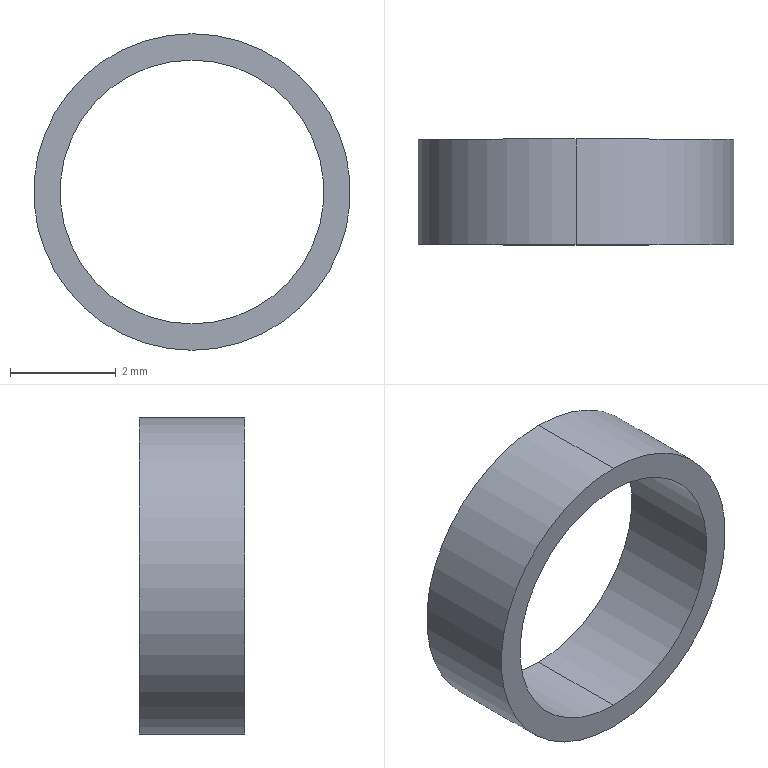Part | SolidWorks | features Extrusion 1 | 1 solid | 6 faces | box 6 x 2 x 6 mm | volume 17.279 mm3 | cylinder 4 | plane 2 | commonest cylinder face diameters 5 x2 6 x2
STEP:
#1=CARTESIAN_POINT('',(0.,2.,-2.5));
#2=VERTEX_POINT('',#1);
#3=CARTESIAN_POINT('',(0.,2.,2.5));
#4=VERTEX_POINT('',#3);
#5=CARTESIAN_POINT('',(0.,2.,0.));
#6=DIRECTION('',(0.,1.,0.));
#7=DIRECTION('',(0.,0.,1.));
#8=AXIS2_PLACEMENT_3D('',#5,#6,#7);
#9=CIRCLE('',#8,2.5);
#10=EDGE_CURVE('',#2,#4,#9,.T.);
#11=ORIENTED_EDGE('',*,*,#10,.T.);
#12=CARTESIAN_POINT('',(0.,0.,2.5));
#13=VERTEX_POINT('',#12);
#14=CARTESIAN_POINT('',(0.,2.,2.5));
#15=DIRECTION('',(0.,-1.,0.));
#16=VECTOR('',#15,1000.);
#17=LINE('',#14,#16);
#18=EDGE_CURVE('',#4,#13,#17,.T.);
#19=ORIENTED_EDGE('',*,*,#18,.T.);
#20=CARTESIAN_POINT('',(0.,0.,-2.5));
#21=VERTEX_POINT('',#20);
#22=CARTESIAN_POINT('',(0.,0.,0.));
#23=DIRECTION('',(0.,1.,0.));
#24=DIRECTION('',(0.,0.,1.));
#25=AXIS2_PLACEMENT_3D('',#22,#23,#24);
#26=CIRCLE('',#25,2.5);
#27=EDGE_CURVE('',#21,#13,#26,.T.);
#28=ORIENTED_EDGE('',*,*,#27,.F.);
#29=CARTESIAN_POINT('',(0.,2.,-2.5));
#30=DIRECTION('',(0.,-1.,0.));
#31=VECTOR('',#30,1000.);
#32=LINE('',#29,#31);
#33=EDGE_CURVE('',#2,#21,#32,.T.);
#34=ORIENTED_EDGE('',*,*,#33,.F.);
#35=EDGE_LOOP('',(#11,#19,#28,#34));
#36=FACE_OUTER_BOUND('',#35,.T.);
#37=CARTESIAN_POINT('',(0.,2.,0.));
#38=DIRECTION('',(0.,-1.,0.));
#39=DIRECTION('',(0.,0.,-1.));
#40=AXIS2_PLACEMENT_3D('',#37,#38,#39);
#41=CYLINDRICAL_SURFACE('',#40,2.5);
#42=ADVANCED_FACE('',(#36),#41,.F.);
#43=CARTESIAN_POINT('',(0.,2.,3.));
#44=VERTEX_POINT('',#43);
#45=CARTESIAN_POINT('',(0.,2.,-3.));
#46=VERTEX_POINT('',#45);
#47=CARTESIAN_POINT('',(0.,2.,0.));
#48=DIRECTION('',(0.,1.,0.));
#49=DIRECTION('',(0.,0.,1.));
#50=AXIS2_PLACEMENT_3D('',#47,#48,#49);
#51=CIRCLE('',#50,3.);
#52=EDGE_CURVE('',#44,#46,#51,.T.);
#53=ORIENTED_EDGE('',*,*,#52,.F.);
#54=CARTESIAN_POINT('',(0.,0.,3.));
#55=VERTEX_POINT('',#54);
#56=CARTESIAN_POINT('',(0.,2.,3.));
#57=DIRECTION('',(0.,-1.,0.));
#58=VECTOR('',#57,1000.);
#59=LINE('',#56,#58);
#60=EDGE_CURVE('',#44,#55,#59,.T.);
#61=ORIENTED_EDGE('',*,*,#60,.T.);
#62=CARTESIAN_POINT('',(0.,0.,-3.));
#63=VERTEX_POINT('',#62);
#64=CARTESIAN_POINT('',(0.,0.,0.));
#65=DIRECTION('',(0.,1.,0.));
#66=DIRECTION('',(0.,0.,1.));
#67=AXIS2_PLACEMENT_3D('',#64,#65,#66);
#68=CIRCLE('',#67,3.);
#69=EDGE_CURVE('',#55,#63,#68,.T.);
#70=ORIENTED_EDGE('',*,*,#69,.T.);
#71=CARTESIAN_POINT('',(0.,2.,-3.));
#72=DIRECTION('',(0.,-1.,0.));
#73=VECTOR('',#72,1000.);
#74=LINE('',#71,#73);
#75=EDGE_CURVE('',#46,#63,#74,.T.);
#76=ORIENTED_EDGE('',*,*,#75,.F.);
#77=EDGE_LOOP('',(#53,#61,#70,#76));
#78=FACE_OUTER_BOUND('',#77,.T.);
#79=CARTESIAN_POINT('',(0.,2.,0.));
#80=DIRECTION('',(0.,-1.,0.));
#81=DIRECTION('',(0.,0.,-1.));
#82=AXIS2_PLACEMENT_3D('',#79,#80,#81);
#83=CYLINDRICAL_SURFACE('',#82,3.);
#84=ADVANCED_FACE('',(#78),#83,.T.);
#85=CARTESIAN_POINT('',(0.,2.,0.));
#86=DIRECTION('',(0.,1.,0.));
#87=DIRECTION('',(0.,0.,1.));
#88=AXIS2_PLACEMENT_3D('',#85,#86,#87);
#89=CIRCLE('',#88,3.);
#90=EDGE_CURVE('',#46,#44,#89,.T.);
#91=ORIENTED_EDGE('',*,*,#90,.T.);
#92=ORIENTED_EDGE('',*,*,#52,.T.);
#93=EDGE_LOOP('',(#91,#92));
#94=FACE_OUTER_BOUND('',#93,.T.);
#95=ORIENTED_EDGE('',*,*,#10,.F.);
#96=CARTESIAN_POINT('',(0.,2.,0.));
#97=DIRECTION('',(0.,1.,0.));
#98=DIRECTION('',(0.,0.,1.));
#99=AXIS2_PLACEMENT_3D('',#96,#97,#98);
#100=CIRCLE('',#99,2.5);
#101=EDGE_CURVE('',#4,#2,#100,.T.);
#102=ORIENTED_EDGE('',*,*,#101,.F.);
#103=EDGE_LOOP('',(#95,#102));
#104=FACE_BOUND('',#103,.T.);
#105=CARTESIAN_POINT('',(0.,2.,0.));
#106=DIRECTION('',(0.,1.,0.));
#107=DIRECTION('',(0.,0.,1.));
#108=AXIS2_PLACEMENT_3D('',#105,#106,#107);
#109=PLANE('',#108);
#110=ADVANCED_FACE('',(#94,#104),#109,.T.);
#111=CARTESIAN_POINT('',(0.,0.,0.));
#112=DIRECTION('',(0.,1.,0.));
#113=DIRECTION('',(0.,0.,1.));
#114=AXIS2_PLACEMENT_3D('',#111,#112,#113);
#115=CIRCLE('',#114,3.);
#116=EDGE_CURVE('',#63,#55,#115,.T.);
#117=ORIENTED_EDGE('',*,*,#116,.F.);
#118=ORIENTED_EDGE('',*,*,#69,.F.);
#119=EDGE_LOOP('',(#117,#118));
#120=FACE_OUTER_BOUND('',#119,.T.);
#121=ORIENTED_EDGE('',*,*,#27,.T.);
#122=CARTESIAN_POINT('',(0.,0.,0.));
#123=DIRECTION('',(0.,1.,0.));
#124=DIRECTION('',(0.,0.,1.));
#125=AXIS2_PLACEMENT_3D('',#122,#123,#124);
#126=CIRCLE('',#125,2.5);
#127=EDGE_CURVE('',#13,#21,#126,.T.);
#128=ORIENTED_EDGE('',*,*,#127,.T.);
#129=EDGE_LOOP('',(#121,#128));
#130=FACE_BOUND('',#129,.T.);
#131=CARTESIAN_POINT('',(0.,0.,0.));
#132=DIRECTION('',(0.,1.,0.));
#133=DIRECTION('',(0.,0.,1.));
#134=AXIS2_PLACEMENT_3D('',#131,#132,#133);
#135=PLANE('',#134);
#136=ADVANCED_FACE('',(#120,#130),#135,.F.);
#137=ORIENTED_EDGE('',*,*,#60,.F.);
#138=ORIENTED_EDGE('',*,*,#90,.F.);
#139=ORIENTED_EDGE('',*,*,#75,.T.);
#140=ORIENTED_EDGE('',*,*,#116,.T.);
#141=EDGE_LOOP('',(#137,#138,#139,#140));
#142=FACE_OUTER_BOUND('',#141,.T.);
#143=CARTESIAN_POINT('',(0.,2.,0.));
#144=DIRECTION('',(0.,-1.,0.));
#145=DIRECTION('',(0.,0.,-1.));
#146=AXIS2_PLACEMENT_3D('',#143,#144,#145);
#147=CYLINDRICAL_SURFACE('',#146,3.);
#148=ADVANCED_FACE('',(#142),#147,.T.);
#149=ORIENTED_EDGE('',*,*,#18,.F.);
#150=ORIENTED_EDGE('',*,*,#101,.T.);
#151=ORIENTED_EDGE('',*,*,#33,.T.);
#152=ORIENTED_EDGE('',*,*,#127,.F.);
#153=EDGE_LOOP('',(#149,#150,#151,#152));
#154=FACE_OUTER_BOUND('',#153,.T.);
#155=CARTESIAN_POINT('',(0.,2.,0.));
#156=DIRECTION('',(0.,-1.,0.));
#157=DIRECTION('',(0.,0.,-1.));
#158=AXIS2_PLACEMENT_3D('',#155,#156,#157);
#159=CYLINDRICAL_SURFACE('',#158,2.5);
#160=ADVANCED_FACE('',(#154),#159,.F.);
#161=CLOSED_SHELL('',(#42,#84,#110,#136,#148,#160));
#162=MANIFOLD_SOLID_BREP('',#161);
#163=CARTESIAN_POINT('',(0.,0.,0.));
#164=DIRECTION('',(0.,0.,1.));
#165=DIRECTION('',(1.,0.,0.));
#166=AXIS2_PLACEMENT_3D('',#163,#164,#165);
#167=(LENGTH_UNIT()NAMED_UNIT(*)SI_UNIT(.MILLI.,.METRE.));
#168=UNCERTAINTY_MEASURE_WITH_UNIT(LENGTH_MEASURE(0.00001),#167,'','');
#169=(NAMED_UNIT(*)PLANE_ANGLE_UNIT()SI_UNIT($,.RADIAN.));
#170=(NAMED_UNIT(*)SI_UNIT($,.STERADIAN.)SOLID_ANGLE_UNIT());
#171=(GEOMETRIC_REPRESENTATION_CONTEXT(3)GLOBAL_UNCERTAINTY_ASSIGNED_CONTEXT((#168))GLOBAL_UNIT_ASSIGNED_CONTEXT((#167,#169,#170))REPRESENTATION_CONTEXT('',''));
#172=ADVANCED_BREP_SHAPE_REPRESENTATION('',(#162,#166),#171);